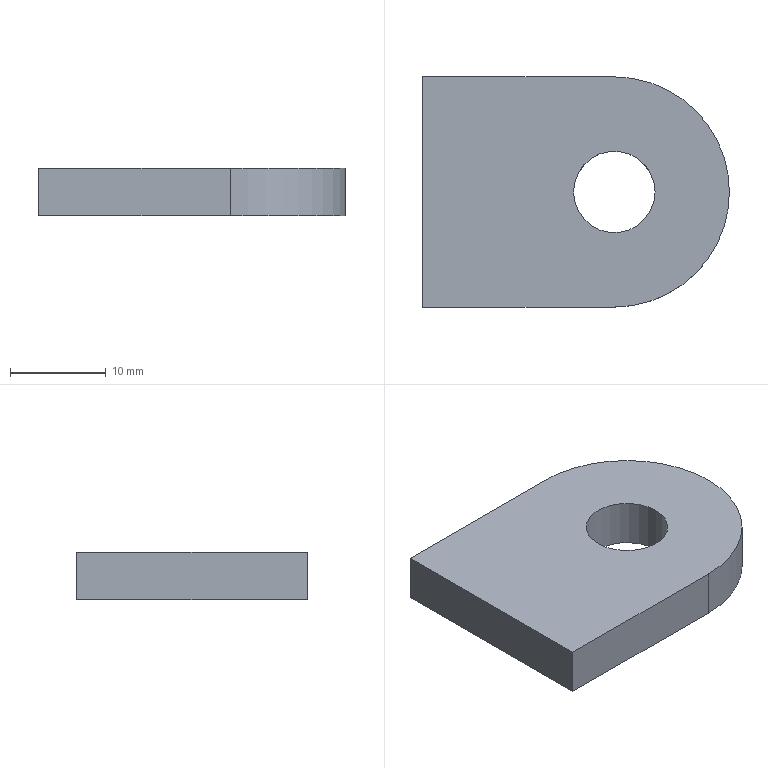Part | NX | features DATUM_CSYS 1, EXTRUDE 1, LINKED_FACE 1, SKETCH 1 | 1 solid | 7 faces | box 32 x 24 x 5 mm | volume 3247 mm3 | plane 5 | cylinder 2 | commonest cylinder face diameters 8.5 x1 24 x1
STEP:
#1=CARTESIAN_POINT('',(20.,12.,5.));
#2=VERTEX_POINT('',#1);
#3=CARTESIAN_POINT('',(20.,-12.,5.));
#4=VERTEX_POINT('',#3);
#5=CARTESIAN_POINT('',(20.,12.,5.));
#6=DIRECTION('',(0.,-1.,0.));
#7=VECTOR('',#6,1000.);
#8=LINE('',#5,#7);
#9=EDGE_CURVE('',#2,#4,#8,.T.);
#10=ORIENTED_EDGE('',*,*,#9,.F.);
#11=CARTESIAN_POINT('',(20.,12.,0.));
#12=VERTEX_POINT('',#11);
#13=CARTESIAN_POINT('',(20.,12.,0.));
#14=DIRECTION('',(0.,0.,1.));
#15=VECTOR('',#14,1000.);
#16=LINE('',#13,#15);
#17=EDGE_CURVE('',#12,#2,#16,.T.);
#18=ORIENTED_EDGE('',*,*,#17,.F.);
#19=CARTESIAN_POINT('',(20.,-12.,0.));
#20=VERTEX_POINT('',#19);
#21=CARTESIAN_POINT('',(20.,12.,0.));
#22=DIRECTION('',(0.,-1.,0.));
#23=VECTOR('',#22,1000.);
#24=LINE('',#21,#23);
#25=EDGE_CURVE('',#12,#20,#24,.T.);
#26=ORIENTED_EDGE('',*,*,#25,.T.);
#27=CARTESIAN_POINT('',(20.,-12.,0.));
#28=DIRECTION('',(0.,0.,1.));
#29=VECTOR('',#28,1000.);
#30=LINE('',#27,#29);
#31=EDGE_CURVE('',#20,#4,#30,.T.);
#32=ORIENTED_EDGE('',*,*,#31,.T.);
#33=EDGE_LOOP('',(#10,#18,#26,#32));
#34=FACE_BOUND('',#33,.T.);
#35=CARTESIAN_POINT('',(20.,12.,0.));
#36=DIRECTION('',(-1.,0.,0.));
#37=DIRECTION('',(0.,0.,1.));
#38=AXIS2_PLACEMENT_3D('',#35,#36,#37);
#39=PLANE('',#38);
#40=ADVANCED_FACE('',(#34),#39,.T.);
#41=CARTESIAN_POINT('',(40.,-12.,5.));
#42=VERTEX_POINT('',#41);
#43=CARTESIAN_POINT('',(20.,-12.,5.));
#44=DIRECTION('',(1.,0.,0.));
#45=VECTOR('',#44,1000.);
#46=LINE('',#43,#45);
#47=EDGE_CURVE('',#4,#42,#46,.T.);
#48=ORIENTED_EDGE('',*,*,#47,.F.);
#49=ORIENTED_EDGE('',*,*,#31,.F.);
#50=CARTESIAN_POINT('',(40.,-12.,0.));
#51=VERTEX_POINT('',#50);
#52=CARTESIAN_POINT('',(20.,-12.,0.));
#53=DIRECTION('',(1.,0.,0.));
#54=VECTOR('',#53,1000.);
#55=LINE('',#52,#54);
#56=EDGE_CURVE('',#20,#51,#55,.T.);
#57=ORIENTED_EDGE('',*,*,#56,.T.);
#58=CARTESIAN_POINT('',(40.,-12.,0.));
#59=DIRECTION('',(0.,0.,1.));
#60=VECTOR('',#59,1000.);
#61=LINE('',#58,#60);
#62=EDGE_CURVE('',#51,#42,#61,.T.);
#63=ORIENTED_EDGE('',*,*,#62,.T.);
#64=EDGE_LOOP('',(#48,#49,#57,#63));
#65=FACE_BOUND('',#64,.T.);
#66=CARTESIAN_POINT('',(20.,-12.,0.));
#67=DIRECTION('',(0.,-1.,0.));
#68=DIRECTION('',(0.,0.,-1.));
#69=AXIS2_PLACEMENT_3D('',#66,#67,#68);
#70=PLANE('',#69);
#71=ADVANCED_FACE('',(#65),#70,.T.);
#72=CARTESIAN_POINT('',(40.,12.,5.));
#73=VERTEX_POINT('',#72);
#74=CARTESIAN_POINT('',(40.,0.,5.));
#75=DIRECTION('',(0.,0.,1.));
#76=DIRECTION('',(0.,-1.,0.));
#77=AXIS2_PLACEMENT_3D('',#74,#75,#76);
#78=CIRCLE('',#77,12.);
#79=EDGE_CURVE('',#42,#73,#78,.T.);
#80=ORIENTED_EDGE('',*,*,#79,.F.);
#81=ORIENTED_EDGE('',*,*,#62,.F.);
#82=CARTESIAN_POINT('',(40.,12.,0.));
#83=VERTEX_POINT('',#82);
#84=CARTESIAN_POINT('',(40.,0.,0.));
#85=DIRECTION('',(0.,0.,1.));
#86=DIRECTION('',(0.,-1.,0.));
#87=AXIS2_PLACEMENT_3D('',#84,#85,#86);
#88=CIRCLE('',#87,12.);
#89=EDGE_CURVE('',#51,#83,#88,.T.);
#90=ORIENTED_EDGE('',*,*,#89,.T.);
#91=CARTESIAN_POINT('',(40.,12.,0.));
#92=DIRECTION('',(0.,0.,1.));
#93=VECTOR('',#92,1000.);
#94=LINE('',#91,#93);
#95=EDGE_CURVE('',#83,#73,#94,.T.);
#96=ORIENTED_EDGE('',*,*,#95,.T.);
#97=EDGE_LOOP('',(#80,#81,#90,#96));
#98=FACE_BOUND('',#97,.T.);
#99=CARTESIAN_POINT('',(40.,0.,0.));
#100=DIRECTION('',(0.,0.,1.));
#101=DIRECTION('',(1.,0.,0.));
#102=AXIS2_PLACEMENT_3D('',#99,#100,#101);
#103=CYLINDRICAL_SURFACE('',#102,12.);
#104=ADVANCED_FACE('',(#98),#103,.T.);
#105=CARTESIAN_POINT('',(40.,12.,5.));
#106=DIRECTION('',(-1.,0.,0.));
#107=VECTOR('',#106,1000.);
#108=LINE('',#105,#107);
#109=EDGE_CURVE('',#73,#2,#108,.T.);
#110=ORIENTED_EDGE('',*,*,#109,.F.);
#111=ORIENTED_EDGE('',*,*,#95,.F.);
#112=CARTESIAN_POINT('',(40.,12.,0.));
#113=DIRECTION('',(-1.,0.,0.));
#114=VECTOR('',#113,1000.);
#115=LINE('',#112,#114);
#116=EDGE_CURVE('',#83,#12,#115,.T.);
#117=ORIENTED_EDGE('',*,*,#116,.T.);
#118=ORIENTED_EDGE('',*,*,#17,.T.);
#119=EDGE_LOOP('',(#110,#111,#117,#118));
#120=FACE_BOUND('',#119,.T.);
#121=CARTESIAN_POINT('',(40.,12.,0.));
#122=DIRECTION('',(0.,1.,0.));
#123=DIRECTION('',(0.,0.,1.));
#124=AXIS2_PLACEMENT_3D('',#121,#122,#123);
#125=PLANE('',#124);
#126=ADVANCED_FACE('',(#120),#125,.T.);
#127=CARTESIAN_POINT('',(35.75,0.,5.));
#128=VERTEX_POINT('',#127);
#129=CARTESIAN_POINT('',(40.,0.,5.));
#130=DIRECTION('',(0.,0.,-1.));
#131=DIRECTION('',(-1.,0.,0.));
#132=AXIS2_PLACEMENT_3D('',#129,#130,#131);
#133=CIRCLE('',#132,4.25);
#134=EDGE_CURVE('',#128,#128,#133,.T.);
#135=ORIENTED_EDGE('',*,*,#134,.F.);
#136=EDGE_LOOP('',(#135));
#137=FACE_BOUND('',#136,.T.);
#138=CARTESIAN_POINT('',(44.25,0.,0.));
#139=VERTEX_POINT('',#138);
#140=CARTESIAN_POINT('',(40.,0.,0.));
#141=DIRECTION('',(0.,0.,-1.));
#142=DIRECTION('',(1.,0.,0.));
#143=AXIS2_PLACEMENT_3D('',#140,#141,#142);
#144=CIRCLE('',#143,4.25);
#145=EDGE_CURVE('',#139,#139,#144,.T.);
#146=ORIENTED_EDGE('',*,*,#145,.T.);
#147=EDGE_LOOP('',(#146));
#148=FACE_BOUND('',#147,.T.);
#149=CARTESIAN_POINT('',(40.,0.,0.));
#150=DIRECTION('',(0.,0.,1.));
#151=DIRECTION('',(1.,0.,0.));
#152=AXIS2_PLACEMENT_3D('',#149,#150,#151);
#153=CYLINDRICAL_SURFACE('',#152,4.25);
#154=ADVANCED_FACE('',(#137,#148),#153,.F.);
#155=ORIENTED_EDGE('',*,*,#25,.F.);
#156=ORIENTED_EDGE('',*,*,#116,.F.);
#157=ORIENTED_EDGE('',*,*,#89,.F.);
#158=ORIENTED_EDGE('',*,*,#56,.F.);
#159=EDGE_LOOP('',(#155,#156,#157,#158));
#160=FACE_BOUND('',#159,.T.);
#161=ORIENTED_EDGE('',*,*,#145,.F.);
#162=EDGE_LOOP('',(#161));
#163=FACE_BOUND('',#162,.T.);
#164=CARTESIAN_POINT('',(40.,0.,0.));
#165=DIRECTION('',(0.,0.,1.));
#166=DIRECTION('',(1.,0.,0.));
#167=AXIS2_PLACEMENT_3D('',#164,#165,#166);
#168=PLANE('',#167);
#169=ADVANCED_FACE('',(#160,#163),#168,.F.);
#170=ORIENTED_EDGE('',*,*,#9,.T.);
#171=ORIENTED_EDGE('',*,*,#47,.T.);
#172=ORIENTED_EDGE('',*,*,#79,.T.);
#173=ORIENTED_EDGE('',*,*,#109,.T.);
#174=EDGE_LOOP('',(#170,#171,#172,#173));
#175=FACE_BOUND('',#174,.T.);
#176=ORIENTED_EDGE('',*,*,#134,.T.);
#177=EDGE_LOOP('',(#176));
#178=FACE_BOUND('',#177,.T.);
#179=CARTESIAN_POINT('',(40.,0.,5.));
#180=DIRECTION('',(0.,0.,1.));
#181=DIRECTION('',(1.,0.,0.));
#182=AXIS2_PLACEMENT_3D('',#179,#180,#181);
#183=PLANE('',#182);
#184=ADVANCED_FACE('',(#175,#178),#183,.T.);
#185=CLOSED_SHELL('',(#40,#71,#104,#126,#154,#169,#184));
#186=MANIFOLD_SOLID_BREP('',#185);
#187=(LENGTH_UNIT()NAMED_UNIT(*)SI_UNIT(.MILLI.,.METRE.));
#188=UNCERTAINTY_MEASURE_WITH_UNIT(LENGTH_MEASURE(0.00001),#187,'','');
#189=(NAMED_UNIT(*)PLANE_ANGLE_UNIT()SI_UNIT($,.RADIAN.));
#190=(NAMED_UNIT(*)SI_UNIT($,.STERADIAN.)SOLID_ANGLE_UNIT());
#191=(GEOMETRIC_REPRESENTATION_CONTEXT(3)GLOBAL_UNCERTAINTY_ASSIGNED_CONTEXT((#188))GLOBAL_UNIT_ASSIGNED_CONTEXT((#187,#189,#190))REPRESENTATION_CONTEXT('',''));
#192=ADVANCED_BREP_SHAPE_REPRESENTATION('',(#186),#191);